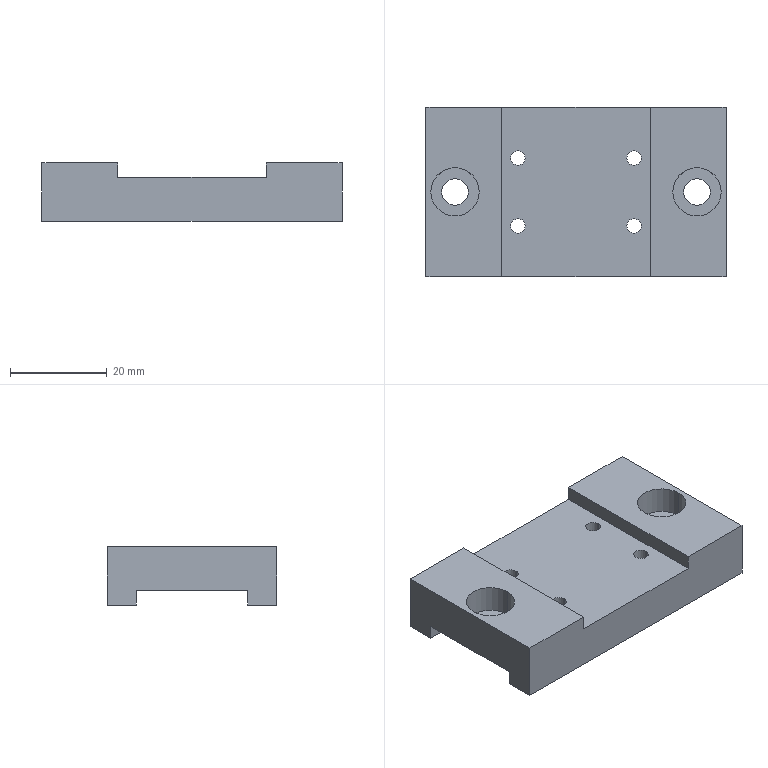Part | STEP file | X77-02302 | 1 solid | 32 faces | box 62 x 35 x 12 mm | volume 17327 mm3 | cylinder 16 | plane 16 | commonest cylinder face diameters 3 x8 5.5 x4 10 x4
STEP:
#1=CARTESIAN_POINT('',(-360.426,46.806,6.3));
#2=VERTEX_POINT('',#1);
#3=CARTESIAN_POINT('',(-350.426,46.806,6.3));
#4=VERTEX_POINT('',#3);
#5=CARTESIAN_POINT('',(-355.426,46.806,6.3));
#6=DIRECTION('',(0.,0.,1.));
#7=DIRECTION('',(1.,0.,0.));
#8=AXIS2_PLACEMENT_3D('',#5,#6,#7);
#9=CIRCLE('',#8,5.);
#10=EDGE_CURVE('',#2,#4,#9,.T.);
#11=ORIENTED_EDGE('',*,*,#10,.F.);
#12=CARTESIAN_POINT('',(-360.426,46.806,12.));
#13=VERTEX_POINT('',#12);
#14=CARTESIAN_POINT('',(-360.426,46.806,12.));
#15=DIRECTION('',(0.,0.,1.));
#16=VECTOR('',#15,1000.);
#17=LINE('',#14,#16);
#18=EDGE_CURVE('',#2,#13,#17,.T.);
#19=ORIENTED_EDGE('',*,*,#18,.T.);
#20=CARTESIAN_POINT('',(-350.426,46.806,12.));
#21=VERTEX_POINT('',#20);
#22=CARTESIAN_POINT('',(-355.426,46.806,12.));
#23=DIRECTION('',(0.,0.,1.));
#24=DIRECTION('',(1.,0.,0.));
#25=AXIS2_PLACEMENT_3D('',#22,#23,#24);
#26=CIRCLE('',#25,5.);
#27=EDGE_CURVE('',#13,#21,#26,.T.);
#28=ORIENTED_EDGE('',*,*,#27,.T.);
#29=CARTESIAN_POINT('',(-350.426,46.806,12.));
#30=DIRECTION('',(0.,0.,1.));
#31=VECTOR('',#30,1000.);
#32=LINE('',#29,#31);
#33=EDGE_CURVE('',#4,#21,#32,.T.);
#34=ORIENTED_EDGE('',*,*,#33,.F.);
#35=EDGE_LOOP('',(#11,#19,#28,#34));
#36=FACE_OUTER_BOUND('',#35,.T.);
#37=CARTESIAN_POINT('',(-355.426,46.806,12.));
#38=DIRECTION('',(0.,0.,1.));
#39=DIRECTION('',(1.,0.,0.));
#40=AXIS2_PLACEMENT_3D('',#37,#38,#39);
#41=CYLINDRICAL_SURFACE('',#40,5.);
#42=ADVANCED_FACE('',(#36),#41,.F.);
#43=CARTESIAN_POINT('',(-358.176,46.806,3.));
#44=VERTEX_POINT('',#43);
#45=CARTESIAN_POINT('',(-352.676,46.806,3.));
#46=VERTEX_POINT('',#45);
#47=CARTESIAN_POINT('',(-355.426,46.806,3.));
#48=DIRECTION('',(0.,0.,1.));
#49=DIRECTION('',(1.,0.,0.));
#50=AXIS2_PLACEMENT_3D('',#47,#48,#49);
#51=CIRCLE('',#50,2.75);
#52=EDGE_CURVE('',#44,#46,#51,.T.);
#53=ORIENTED_EDGE('',*,*,#52,.F.);
#54=CARTESIAN_POINT('',(-358.176,46.806,6.3));
#55=VERTEX_POINT('',#54);
#56=CARTESIAN_POINT('',(-358.176,46.806,12.));
#57=DIRECTION('',(0.,0.,1.));
#58=VECTOR('',#57,1000.);
#59=LINE('',#56,#58);
#60=EDGE_CURVE('',#44,#55,#59,.T.);
#61=ORIENTED_EDGE('',*,*,#60,.T.);
#62=CARTESIAN_POINT('',(-352.676,46.806,6.3));
#63=VERTEX_POINT('',#62);
#64=CARTESIAN_POINT('',(-355.426,46.806,6.3));
#65=DIRECTION('',(0.,0.,1.));
#66=DIRECTION('',(1.,0.,0.));
#67=AXIS2_PLACEMENT_3D('',#64,#65,#66);
#68=CIRCLE('',#67,2.75);
#69=EDGE_CURVE('',#55,#63,#68,.T.);
#70=ORIENTED_EDGE('',*,*,#69,.T.);
#71=CARTESIAN_POINT('',(-352.676,46.806,12.));
#72=DIRECTION('',(0.,0.,1.));
#73=VECTOR('',#72,1000.);
#74=LINE('',#71,#73);
#75=EDGE_CURVE('',#46,#63,#74,.T.);
#76=ORIENTED_EDGE('',*,*,#75,.F.);
#77=EDGE_LOOP('',(#53,#61,#70,#76));
#78=FACE_OUTER_BOUND('',#77,.T.);
#79=CARTESIAN_POINT('',(-355.426,46.806,12.));
#80=DIRECTION('',(0.,0.,1.));
#81=DIRECTION('',(1.,0.,0.));
#82=AXIS2_PLACEMENT_3D('',#79,#80,#81);
#83=CYLINDRICAL_SURFACE('',#82,2.75);
#84=ADVANCED_FACE('',(#78),#83,.F.);
#85=CARTESIAN_POINT('',(-310.426,46.806,6.3));
#86=VERTEX_POINT('',#85);
#87=CARTESIAN_POINT('',(-300.426,46.806,6.3));
#88=VERTEX_POINT('',#87);
#89=CARTESIAN_POINT('',(-305.426,46.806,6.3));
#90=DIRECTION('',(0.,0.,1.));
#91=DIRECTION('',(1.,0.,0.));
#92=AXIS2_PLACEMENT_3D('',#89,#90,#91);
#93=CIRCLE('',#92,5.);
#94=EDGE_CURVE('',#86,#88,#93,.T.);
#95=ORIENTED_EDGE('',*,*,#94,.F.);
#96=CARTESIAN_POINT('',(-310.426,46.806,12.));
#97=VERTEX_POINT('',#96);
#98=CARTESIAN_POINT('',(-310.426,46.806,12.));
#99=DIRECTION('',(0.,0.,1.));
#100=VECTOR('',#99,1000.);
#101=LINE('',#98,#100);
#102=EDGE_CURVE('',#86,#97,#101,.T.);
#103=ORIENTED_EDGE('',*,*,#102,.T.);
#104=CARTESIAN_POINT('',(-300.426,46.806,12.));
#105=VERTEX_POINT('',#104);
#106=CARTESIAN_POINT('',(-305.426,46.806,12.));
#107=DIRECTION('',(0.,0.,1.));
#108=DIRECTION('',(1.,0.,0.));
#109=AXIS2_PLACEMENT_3D('',#106,#107,#108);
#110=CIRCLE('',#109,5.);
#111=EDGE_CURVE('',#97,#105,#110,.T.);
#112=ORIENTED_EDGE('',*,*,#111,.T.);
#113=CARTESIAN_POINT('',(-300.426,46.806,12.));
#114=DIRECTION('',(0.,0.,1.));
#115=VECTOR('',#114,1000.);
#116=LINE('',#113,#115);
#117=EDGE_CURVE('',#88,#105,#116,.T.);
#118=ORIENTED_EDGE('',*,*,#117,.F.);
#119=EDGE_LOOP('',(#95,#103,#112,#118));
#120=FACE_OUTER_BOUND('',#119,.T.);
#121=CARTESIAN_POINT('',(-305.426,46.806,12.));
#122=DIRECTION('',(0.,0.,1.));
#123=DIRECTION('',(1.,0.,0.));
#124=AXIS2_PLACEMENT_3D('',#121,#122,#123);
#125=CYLINDRICAL_SURFACE('',#124,5.);
#126=ADVANCED_FACE('',(#120),#125,.F.);
#127=CARTESIAN_POINT('',(-308.176,46.806,3.));
#128=VERTEX_POINT('',#127);
#129=CARTESIAN_POINT('',(-302.676,46.806,3.));
#130=VERTEX_POINT('',#129);
#131=CARTESIAN_POINT('',(-305.426,46.806,3.));
#132=DIRECTION('',(0.,0.,1.));
#133=DIRECTION('',(1.,0.,0.));
#134=AXIS2_PLACEMENT_3D('',#131,#132,#133);
#135=CIRCLE('',#134,2.75);
#136=EDGE_CURVE('',#128,#130,#135,.T.);
#137=ORIENTED_EDGE('',*,*,#136,.F.);
#138=CARTESIAN_POINT('',(-308.176,46.806,6.3));
#139=VERTEX_POINT('',#138);
#140=CARTESIAN_POINT('',(-308.176,46.806,12.));
#141=DIRECTION('',(0.,0.,1.));
#142=VECTOR('',#141,1000.);
#143=LINE('',#140,#142);
#144=EDGE_CURVE('',#128,#139,#143,.T.);
#145=ORIENTED_EDGE('',*,*,#144,.T.);
#146=CARTESIAN_POINT('',(-302.676,46.806,6.3));
#147=VERTEX_POINT('',#146);
#148=CARTESIAN_POINT('',(-305.426,46.806,6.3));
#149=DIRECTION('',(0.,0.,1.));
#150=DIRECTION('',(1.,0.,0.));
#151=AXIS2_PLACEMENT_3D('',#148,#149,#150);
#152=CIRCLE('',#151,2.75);
#153=EDGE_CURVE('',#139,#147,#152,.T.);
#154=ORIENTED_EDGE('',*,*,#153,.T.);
#155=CARTESIAN_POINT('',(-302.676,46.806,12.));
#156=DIRECTION('',(0.,0.,1.));
#157=VECTOR('',#156,1000.);
#158=LINE('',#155,#157);
#159=EDGE_CURVE('',#130,#147,#158,.T.);
#160=ORIENTED_EDGE('',*,*,#159,.F.);
#161=EDGE_LOOP('',(#137,#145,#154,#160));
#162=FACE_OUTER_BOUND('',#161,.T.);
#163=CARTESIAN_POINT('',(-305.426,46.806,12.));
#164=DIRECTION('',(0.,0.,1.));
#165=DIRECTION('',(1.,0.,0.));
#166=AXIS2_PLACEMENT_3D('',#163,#164,#165);
#167=CYLINDRICAL_SURFACE('',#166,2.75);
#168=ADVANCED_FACE('',(#162),#167,.F.);
#169=CARTESIAN_POINT('',(-319.926,53.806,3.));
#170=VERTEX_POINT('',#169);
#171=CARTESIAN_POINT('',(-316.926,53.806,3.));
#172=VERTEX_POINT('',#171);
#173=CARTESIAN_POINT('',(-318.426,53.806,3.));
#174=DIRECTION('',(0.,0.,1.));
#175=DIRECTION('',(1.,0.,0.));
#176=AXIS2_PLACEMENT_3D('',#173,#174,#175);
#177=CIRCLE('',#176,1.5);
#178=EDGE_CURVE('',#170,#172,#177,.T.);
#179=ORIENTED_EDGE('',*,*,#178,.F.);
#180=CARTESIAN_POINT('',(-319.926,53.806,9.));
#181=VERTEX_POINT('',#180);
#182=CARTESIAN_POINT('',(-319.926,53.806,12.));
#183=DIRECTION('',(0.,0.,1.));
#184=VECTOR('',#183,1000.);
#185=LINE('',#182,#184);
#186=EDGE_CURVE('',#170,#181,#185,.T.);
#187=ORIENTED_EDGE('',*,*,#186,.T.);
#188=CARTESIAN_POINT('',(-316.926,53.806,9.));
#189=VERTEX_POINT('',#188);
#190=CARTESIAN_POINT('',(-318.426,53.806,9.));
#191=DIRECTION('',(0.,0.,1.));
#192=DIRECTION('',(1.,0.,0.));
#193=AXIS2_PLACEMENT_3D('',#190,#191,#192);
#194=CIRCLE('',#193,1.5);
#195=EDGE_CURVE('',#181,#189,#194,.T.);
#196=ORIENTED_EDGE('',*,*,#195,.T.);
#197=CARTESIAN_POINT('',(-316.926,53.806,12.));
#198=DIRECTION('',(0.,0.,1.));
#199=VECTOR('',#198,1000.);
#200=LINE('',#197,#199);
#201=EDGE_CURVE('',#172,#189,#200,.T.);
#202=ORIENTED_EDGE('',*,*,#201,.F.);
#203=EDGE_LOOP('',(#179,#187,#196,#202));
#204=FACE_OUTER_BOUND('',#203,.T.);
#205=CARTESIAN_POINT('',(-318.426,53.806,12.));
#206=DIRECTION('',(0.,0.,1.));
#207=DIRECTION('',(1.,0.,0.));
#208=AXIS2_PLACEMENT_3D('',#205,#206,#207);
#209=CYLINDRICAL_SURFACE('',#208,1.5);
#210=ADVANCED_FACE('',(#204),#209,.F.);
#211=CARTESIAN_POINT('',(-343.926,53.806,3.));
#212=VERTEX_POINT('',#211);
#213=CARTESIAN_POINT('',(-340.926,53.806,3.));
#214=VERTEX_POINT('',#213);
#215=CARTESIAN_POINT('',(-342.426,53.806,3.));
#216=DIRECTION('',(0.,0.,1.));
#217=DIRECTION('',(1.,0.,0.));
#218=AXIS2_PLACEMENT_3D('',#215,#216,#217);
#219=CIRCLE('',#218,1.5);
#220=EDGE_CURVE('',#212,#214,#219,.T.);
#221=ORIENTED_EDGE('',*,*,#220,.F.);
#222=CARTESIAN_POINT('',(-343.926,53.806,9.));
#223=VERTEX_POINT('',#222);
#224=CARTESIAN_POINT('',(-343.926,53.806,12.));
#225=DIRECTION('',(0.,0.,1.));
#226=VECTOR('',#225,1000.);
#227=LINE('',#224,#226);
#228=EDGE_CURVE('',#212,#223,#227,.T.);
#229=ORIENTED_EDGE('',*,*,#228,.T.);
#230=CARTESIAN_POINT('',(-340.926,53.806,9.));
#231=VERTEX_POINT('',#230);
#232=CARTESIAN_POINT('',(-342.426,53.806,9.));
#233=DIRECTION('',(0.,0.,1.));
#234=DIRECTION('',(1.,0.,0.));
#235=AXIS2_PLACEMENT_3D('',#232,#233,#234);
#236=CIRCLE('',#235,1.5);
#237=EDGE_CURVE('',#223,#231,#236,.T.);
#238=ORIENTED_EDGE('',*,*,#237,.T.);
#239=CARTESIAN_POINT('',(-340.926,53.806,12.));
#240=DIRECTION('',(0.,0.,1.));
#241=VECTOR('',#240,1000.);
#242=LINE('',#239,#241);
#243=EDGE_CURVE('',#214,#231,#242,.T.);
#244=ORIENTED_EDGE('',*,*,#243,.F.);
#245=EDGE_LOOP('',(#221,#229,#238,#244));
#246=FACE_OUTER_BOUND('',#245,.T.);
#247=CARTESIAN_POINT('',(-342.426,53.806,12.));
#248=DIRECTION('',(0.,0.,1.));
#249=DIRECTION('',(1.,0.,0.));
#250=AXIS2_PLACEMENT_3D('',#247,#248,#249);
#251=CYLINDRICAL_SURFACE('',#250,1.5);
#252=ADVANCED_FACE('',(#246),#251,.F.);
#253=CARTESIAN_POINT('',(-319.926,39.806,3.));
#254=VERTEX_POINT('',#253);
#255=CARTESIAN_POINT('',(-316.926,39.806,3.));
#256=VERTEX_POINT('',#255);
#257=CARTESIAN_POINT('',(-318.426,39.806,3.));
#258=DIRECTION('',(0.,0.,1.));
#259=DIRECTION('',(1.,0.,0.));
#260=AXIS2_PLACEMENT_3D('',#257,#258,#259);
#261=CIRCLE('',#260,1.5);
#262=EDGE_CURVE('',#254,#256,#261,.T.);
#263=ORIENTED_EDGE('',*,*,#262,.F.);
#264=CARTESIAN_POINT('',(-319.926,39.806,9.));
#265=VERTEX_POINT('',#264);
#266=CARTESIAN_POINT('',(-319.926,39.806,12.));
#267=DIRECTION('',(0.,0.,1.));
#268=VECTOR('',#267,1000.);
#269=LINE('',#266,#268);
#270=EDGE_CURVE('',#254,#265,#269,.T.);
#271=ORIENTED_EDGE('',*,*,#270,.T.);
#272=CARTESIAN_POINT('',(-316.926,39.806,9.));
#273=VERTEX_POINT('',#272);
#274=CARTESIAN_POINT('',(-318.426,39.806,9.));
#275=DIRECTION('',(0.,0.,1.));
#276=DIRECTION('',(1.,0.,0.));
#277=AXIS2_PLACEMENT_3D('',#274,#275,#276);
#278=CIRCLE('',#277,1.5);
#279=EDGE_CURVE('',#265,#273,#278,.T.);
#280=ORIENTED_EDGE('',*,*,#279,.T.);
#281=CARTESIAN_POINT('',(-316.926,39.806,12.));
#282=DIRECTION('',(0.,0.,1.));
#283=VECTOR('',#282,1000.);
#284=LINE('',#281,#283);
#285=EDGE_CURVE('',#256,#273,#284,.T.);
#286=ORIENTED_EDGE('',*,*,#285,.F.);
#287=EDGE_LOOP('',(#263,#271,#280,#286));
#288=FACE_OUTER_BOUND('',#287,.T.);
#289=CARTESIAN_POINT('',(-318.426,39.806,12.));
#290=DIRECTION('',(0.,0.,1.));
#291=DIRECTION('',(1.,0.,0.));
#292=AXIS2_PLACEMENT_3D('',#289,#290,#291);
#293=CYLINDRICAL_SURFACE('',#292,1.5);
#294=ADVANCED_FACE('',(#288),#293,.F.);
#295=CARTESIAN_POINT('',(-343.926,39.806,3.));
#296=VERTEX_POINT('',#295);
#297=CARTESIAN_POINT('',(-340.926,39.806,3.));
#298=VERTEX_POINT('',#297);
#299=CARTESIAN_POINT('',(-342.426,39.806,3.));
#300=DIRECTION('',(0.,0.,1.));
#301=DIRECTION('',(1.,0.,0.));
#302=AXIS2_PLACEMENT_3D('',#299,#300,#301);
#303=CIRCLE('',#302,1.5);
#304=EDGE_CURVE('',#296,#298,#303,.T.);
#305=ORIENTED_EDGE('',*,*,#304,.F.);
#306=CARTESIAN_POINT('',(-343.926,39.806,9.));
#307=VERTEX_POINT('',#306);
#308=CARTESIAN_POINT('',(-343.926,39.806,12.));
#309=DIRECTION('',(0.,0.,1.));
#310=VECTOR('',#309,1000.);
#311=LINE('',#308,#310);
#312=EDGE_CURVE('',#296,#307,#311,.T.);
#313=ORIENTED_EDGE('',*,*,#312,.T.);
#314=CARTESIAN_POINT('',(-340.926,39.806,9.));
#315=VERTEX_POINT('',#314);
#316=CARTESIAN_POINT('',(-342.426,39.806,9.));
#317=DIRECTION('',(0.,0.,1.));
#318=DIRECTION('',(1.,0.,0.));
#319=AXIS2_PLACEMENT_3D('',#316,#317,#318);
#320=CIRCLE('',#319,1.5);
#321=EDGE_CURVE('',#307,#315,#320,.T.);
#322=ORIENTED_EDGE('',*,*,#321,.T.);
#323=CARTESIAN_POINT('',(-340.926,39.806,12.));
#324=DIRECTION('',(0.,0.,1.));
#325=VECTOR('',#324,1000.);
#326=LINE('',#323,#325);
#327=EDGE_CURVE('',#298,#315,#326,.T.);
#328=ORIENTED_EDGE('',*,*,#327,.F.);
#329=EDGE_LOOP('',(#305,#313,#322,#328));
#330=FACE_OUTER_BOUND('',#329,.T.);
#331=CARTESIAN_POINT('',(-342.426,39.806,12.));
#332=DIRECTION('',(0.,0.,1.));
#333=DIRECTION('',(1.,0.,0.));
#334=AXIS2_PLACEMENT_3D('',#331,#332,#333);
#335=CYLINDRICAL_SURFACE('',#334,1.5);
#336=ADVANCED_FACE('',(#330),#335,.F.);
#337=CARTESIAN_POINT('',(-361.426,35.306,0.));
#338=VERTEX_POINT('',#337);
#339=CARTESIAN_POINT('',(-361.426,29.306,0.));
#340=VERTEX_POINT('',#339);
#341=CARTESIAN_POINT('',(-361.426,29.306,0.));
#342=DIRECTION('',(0.,-1.,0.));
#343=VECTOR('',#342,1000.);
#344=LINE('',#341,#343);
#345=EDGE_CURVE('',#338,#340,#344,.T.);
#346=ORIENTED_EDGE('',*,*,#345,.F.);
#347=CARTESIAN_POINT('',(-299.426,35.306,0.));
#348=VERTEX_POINT('',#347);
#349=CARTESIAN_POINT('',(-361.426,35.306,0.));
#350=DIRECTION('',(1.,0.,0.));
#351=VECTOR('',#350,1000.);
#352=LINE('',#349,#351);
#353=EDGE_CURVE('',#338,#348,#352,.T.);
#354=ORIENTED_EDGE('',*,*,#353,.T.);
#355=CARTESIAN_POINT('',(-299.426,29.306,0.));
#356=VERTEX_POINT('',#355);
#357=CARTESIAN_POINT('',(-299.426,29.306,0.));
#358=DIRECTION('',(0.,1.,0.));
#359=VECTOR('',#358,1000.);
#360=LINE('',#357,#359);
#361=EDGE_CURVE('',#356,#348,#360,.T.);
#362=ORIENTED_EDGE('',*,*,#361,.F.);
#363=CARTESIAN_POINT('',(-299.426,29.306,0.));
#364=DIRECTION('',(1.,0.,0.));
#365=VECTOR('',#364,1000.);
#366=LINE('',#363,#365);
#367=EDGE_CURVE('',#340,#356,#366,.T.);
#368=ORIENTED_EDGE('',*,*,#367,.F.);
#369=EDGE_LOOP('',(#346,#354,#362,#368));
#370=FACE_OUTER_BOUND('',#369,.T.);
#371=CARTESIAN_POINT('',(-361.426,64.306,0.));
#372=DIRECTION('',(0.,0.,1.));
#373=DIRECTION('',(1.,0.,0.));
#374=AXIS2_PLACEMENT_3D('',#371,#372,#373);
#375=PLANE('',#374);
#376=ADVANCED_FACE('',(#370),#375,.F.);
#377=CARTESIAN_POINT('',(-305.426,46.806,12.));
#378=DIRECTION('',(0.,0.,1.));
#379=DIRECTION('',(1.,0.,0.));
#380=AXIS2_PLACEMENT_3D('',#377,#378,#379);
#381=CIRCLE('',#380,5.);
#382=EDGE_CURVE('',#105,#97,#381,.T.);
#383=ORIENTED_EDGE('',*,*,#382,.F.);
#384=ORIENTED_EDGE('',*,*,#111,.F.);
#385=EDGE_LOOP('',(#383,#384));
#386=FACE_BOUND('',#385,.T.);
#387=CARTESIAN_POINT('',(-315.126,29.306,12.));
#388=VERTEX_POINT('',#387);
#389=CARTESIAN_POINT('',(-315.126,64.306,12.));
#390=VERTEX_POINT('',#389);
#391=CARTESIAN_POINT('',(-315.126,64.306,12.));
#392=DIRECTION('',(0.,1.,0.));
#393=VECTOR('',#392,1000.);
#394=LINE('',#391,#393);
#395=EDGE_CURVE('',#388,#390,#394,.T.);
#396=ORIENTED_EDGE('',*,*,#395,.F.);
#397=CARTESIAN_POINT('',(-299.426,29.306,12.));
#398=VERTEX_POINT('',#397);
#399=CARTESIAN_POINT('',(-299.426,29.306,12.));
#400=DIRECTION('',(1.,0.,0.));
#401=VECTOR('',#400,1000.);
#402=LINE('',#399,#401);
#403=EDGE_CURVE('',#388,#398,#402,.T.);
#404=ORIENTED_EDGE('',*,*,#403,.T.);
#405=CARTESIAN_POINT('',(-299.426,64.306,12.));
#406=VERTEX_POINT('',#405);
#407=CARTESIAN_POINT('',(-299.426,29.306,12.));
#408=DIRECTION('',(0.,1.,0.));
#409=VECTOR('',#408,1000.);
#410=LINE('',#407,#409);
#411=EDGE_CURVE('',#398,#406,#410,.T.);
#412=ORIENTED_EDGE('',*,*,#411,.T.);
#413=CARTESIAN_POINT('',(-299.426,64.306,12.));
#414=DIRECTION('',(-1.,0.,0.));
#415=VECTOR('',#414,1000.);
#416=LINE('',#413,#415);
#417=EDGE_CURVE('',#406,#390,#416,.T.);
#418=ORIENTED_EDGE('',*,*,#417,.T.);
#419=EDGE_LOOP('',(#396,#404,#412,#418));
#420=FACE_OUTER_BOUND('',#419,.T.);
#421=CARTESIAN_POINT('',(-361.426,64.306,12.));
#422=DIRECTION('',(0.,0.,1.));
#423=DIRECTION('',(1.,0.,0.));
#424=AXIS2_PLACEMENT_3D('',#421,#422,#423);
#425=PLANE('',#424);
#426=ADVANCED_FACE('',(#386,#420),#425,.T.);
#427=CARTESIAN_POINT('',(-361.426,58.306,3.));
#428=VERTEX_POINT('',#427);
#429=CARTESIAN_POINT('',(-361.426,35.306,3.));
#430=VERTEX_POINT('',#429);
#431=CARTESIAN_POINT('',(-361.426,35.306,3.));
#432=DIRECTION('',(0.,-1.,0.));
#433=VECTOR('',#432,1000.);
#434=LINE('',#431,#433);
#435=EDGE_CURVE('',#428,#430,#434,.T.);
#436=ORIENTED_EDGE('',*,*,#435,.T.);
#437=CARTESIAN_POINT('',(-361.426,35.306,0.));
#438=DIRECTION('',(0.,0.,-1.));
#439=VECTOR('',#438,1000.);
#440=LINE('',#437,#439);
#441=EDGE_CURVE('',#430,#338,#440,.T.);
#442=ORIENTED_EDGE('',*,*,#441,.T.);
#443=ORIENTED_EDGE('',*,*,#345,.T.);
#444=CARTESIAN_POINT('',(-361.426,29.306,12.));
#445=VERTEX_POINT('',#444);
#446=CARTESIAN_POINT('',(-361.426,29.306,12.));
#447=DIRECTION('',(0.,0.,-1.));
#448=VECTOR('',#447,1000.);
#449=LINE('',#446,#448);
#450=EDGE_CURVE('',#445,#340,#449,.T.);
#451=ORIENTED_EDGE('',*,*,#450,.F.);
#452=CARTESIAN_POINT('',(-361.426,64.306,12.));
#453=VERTEX_POINT('',#452);
#454=CARTESIAN_POINT('',(-361.426,29.306,12.));
#455=DIRECTION('',(0.,-1.,0.));
#456=VECTOR('',#455,1000.);
#457=LINE('',#454,#456);
#458=EDGE_CURVE('',#453,#445,#457,.T.);
#459=ORIENTED_EDGE('',*,*,#458,.F.);
#460=CARTESIAN_POINT('',(-361.426,64.306,0.));
#461=VERTEX_POINT('',#460);
#462=CARTESIAN_POINT('',(-361.426,64.306,12.));
#463=DIRECTION('',(0.,0.,-1.));
#464=VECTOR('',#463,1000.);
#465=LINE('',#462,#464);
#466=EDGE_CURVE('',#453,#461,#465,.T.);
#467=ORIENTED_EDGE('',*,*,#466,.T.);
#468=CARTESIAN_POINT('',(-361.426,58.306,0.));
#469=VERTEX_POINT('',#468);
#470=CARTESIAN_POINT('',(-361.426,29.306,0.));
#471=DIRECTION('',(0.,-1.,0.));
#472=VECTOR('',#471,1000.);
#473=LINE('',#470,#472);
#474=EDGE_CURVE('',#461,#469,#473,.T.);
#475=ORIENTED_EDGE('',*,*,#474,.T.);
#476=CARTESIAN_POINT('',(-361.426,58.306,0.));
#477=DIRECTION('',(0.,0.,1.));
#478=VECTOR('',#477,1000.);
#479=LINE('',#476,#478);
#480=EDGE_CURVE('',#469,#428,#479,.T.);
#481=ORIENTED_EDGE('',*,*,#480,.T.);
#482=EDGE_LOOP('',(#436,#442,#443,#451,#459,#467,#475,#481));
#483=FACE_OUTER_BOUND('',#482,.T.);
#484=CARTESIAN_POINT('',(-361.426,29.306,12.));
#485=DIRECTION('',(1.,0.,0.));
#486=DIRECTION('',(0.,0.,-1.));
#487=AXIS2_PLACEMENT_3D('',#484,#485,#486);
#488=PLANE('',#487);
#489=ADVANCED_FACE('',(#483),#488,.F.);
#490=ORIENTED_EDGE('',*,*,#403,.F.);
#491=CARTESIAN_POINT('',(-315.126,29.306,9.));
#492=VERTEX_POINT('',#491);
#493=CARTESIAN_POINT('',(-315.126,29.306,12.));
#494=DIRECTION('',(0.,0.,-1.));
#495=VECTOR('',#494,1000.);
#496=LINE('',#493,#495);
#497=EDGE_CURVE('',#388,#492,#496,.T.);
#498=ORIENTED_EDGE('',*,*,#497,.T.);
#499=CARTESIAN_POINT('',(-345.726,29.306,9.));
#500=VERTEX_POINT('',#499);
#501=CARTESIAN_POINT('',(-299.426,29.306,9.));
#502=DIRECTION('',(1.,0.,0.));
#503=VECTOR('',#502,1000.);
#504=LINE('',#501,#503);
#505=EDGE_CURVE('',#500,#492,#504,.T.);
#506=ORIENTED_EDGE('',*,*,#505,.F.);
#507=CARTESIAN_POINT('',(-345.726,29.306,12.));
#508=VERTEX_POINT('',#507);
#509=CARTESIAN_POINT('',(-345.726,29.306,12.));
#510=DIRECTION('',(0.,0.,1.));
#511=VECTOR('',#510,1000.);
#512=LINE('',#509,#511);
#513=EDGE_CURVE('',#500,#508,#512,.T.);
#514=ORIENTED_EDGE('',*,*,#513,.T.);
#515=CARTESIAN_POINT('',(-299.426,29.306,12.));
#516=DIRECTION('',(1.,0.,0.));
#517=VECTOR('',#516,1000.);
#518=LINE('',#515,#517);
#519=EDGE_CURVE('',#445,#508,#518,.T.);
#520=ORIENTED_EDGE('',*,*,#519,.F.);
#521=ORIENTED_EDGE('',*,*,#450,.T.);
#522=ORIENTED_EDGE('',*,*,#367,.T.);
#523=CARTESIAN_POINT('',(-299.426,29.306,12.));
#524=DIRECTION('',(0.,0.,-1.));
#525=VECTOR('',#524,1000.);
#526=LINE('',#523,#525);
#527=EDGE_CURVE('',#398,#356,#526,.T.);
#528=ORIENTED_EDGE('',*,*,#527,.F.);
#529=EDGE_LOOP('',(#490,#498,#506,#514,#520,#521,#522,#528));
#530=FACE_OUTER_BOUND('',#529,.T.);
#531=CARTESIAN_POINT('',(-299.426,29.306,12.));
#532=DIRECTION('',(0.,1.,0.));
#533=DIRECTION('',(-1.,0.,0.));
#534=AXIS2_PLACEMENT_3D('',#531,#532,#533);
#535=PLANE('',#534);
#536=ADVANCED_FACE('',(#530),#535,.F.);
#537=ORIENTED_EDGE('',*,*,#361,.T.);
#538=CARTESIAN_POINT('',(-299.426,35.306,3.));
#539=VERTEX_POINT('',#538);
#540=CARTESIAN_POINT('',(-299.426,35.306,0.));
#541=DIRECTION('',(0.,0.,-1.));
#542=VECTOR('',#541,1000.);
#543=LINE('',#540,#542);
#544=EDGE_CURVE('',#539,#348,#543,.T.);
#545=ORIENTED_EDGE('',*,*,#544,.F.);
#546=CARTESIAN_POINT('',(-299.426,58.306,3.));
#547=VERTEX_POINT('',#546);
#548=CARTESIAN_POINT('',(-299.426,35.306,3.));
#549=DIRECTION('',(0.,-1.,0.));
#550=VECTOR('',#549,1000.);
#551=LINE('',#548,#550);
#552=EDGE_CURVE('',#547,#539,#551,.T.);
#553=ORIENTED_EDGE('',*,*,#552,.F.);
#554=CARTESIAN_POINT('',(-299.426,58.306,0.));
#555=VERTEX_POINT('',#554);
#556=CARTESIAN_POINT('',(-299.426,58.306,0.));
#557=DIRECTION('',(0.,0.,1.));
#558=VECTOR('',#557,1000.);
#559=LINE('',#556,#558);
#560=EDGE_CURVE('',#555,#547,#559,.T.);
#561=ORIENTED_EDGE('',*,*,#560,.F.);
#562=CARTESIAN_POINT('',(-299.426,64.306,0.));
#563=VERTEX_POINT('',#562);
#564=CARTESIAN_POINT('',(-299.426,29.306,0.));
#565=DIRECTION('',(0.,1.,0.));
#566=VECTOR('',#565,1000.);
#567=LINE('',#564,#566);
#568=EDGE_CURVE('',#555,#563,#567,.T.);
#569=ORIENTED_EDGE('',*,*,#568,.T.);
#570=CARTESIAN_POINT('',(-299.426,64.306,12.));
#571=DIRECTION('',(0.,0.,-1.));
#572=VECTOR('',#571,1000.);
#573=LINE('',#570,#572);
#574=EDGE_CURVE('',#406,#563,#573,.T.);
#575=ORIENTED_EDGE('',*,*,#574,.F.);
#576=ORIENTED_EDGE('',*,*,#411,.F.);
#577=ORIENTED_EDGE('',*,*,#527,.T.);
#578=EDGE_LOOP('',(#537,#545,#553,#561,#569,#575,#576,#577));
#579=FACE_OUTER_BOUND('',#578,.T.);
#580=CARTESIAN_POINT('',(-299.426,29.306,12.));
#581=DIRECTION('',(-1.,0.,0.));
#582=DIRECTION('',(0.,0.,1.));
#583=AXIS2_PLACEMENT_3D('',#580,#581,#582);
#584=PLANE('',#583);
#585=ADVANCED_FACE('',(#579),#584,.F.);
#586=CARTESIAN_POINT('',(-315.126,64.306,9.));
#587=VERTEX_POINT('',#586);
#588=CARTESIAN_POINT('',(-345.726,64.306,9.));
#589=VERTEX_POINT('',#588);
#590=CARTESIAN_POINT('',(-299.426,64.306,9.));
#591=DIRECTION('',(-1.,0.,0.));
#592=VECTOR('',#591,1000.);
#593=LINE('',#590,#592);
#594=EDGE_CURVE('',#587,#589,#593,.T.);
#595=ORIENTED_EDGE('',*,*,#594,.F.);
#596=CARTESIAN_POINT('',(-315.126,64.306,12.));
#597=DIRECTION('',(0.,0.,1.));
#598=VECTOR('',#597,1000.);
#599=LINE('',#596,#598);
#600=EDGE_CURVE('',#587,#390,#599,.T.);
#601=ORIENTED_EDGE('',*,*,#600,.T.);
#602=ORIENTED_EDGE('',*,*,#417,.F.);
#603=ORIENTED_EDGE('',*,*,#574,.T.);
#604=CARTESIAN_POINT('',(-299.426,64.306,0.));
#605=DIRECTION('',(-1.,0.,0.));
#606=VECTOR('',#605,1000.);
#607=LINE('',#604,#606);
#608=EDGE_CURVE('',#563,#461,#607,.T.);
#609=ORIENTED_EDGE('',*,*,#608,.T.);
#610=ORIENTED_EDGE('',*,*,#466,.F.);
#611=CARTESIAN_POINT('',(-345.726,64.306,12.));
#612=VERTEX_POINT('',#611);
#613=CARTESIAN_POINT('',(-299.426,64.306,12.));
#614=DIRECTION('',(-1.,0.,0.));
#615=VECTOR('',#614,1000.);
#616=LINE('',#613,#615);
#617=EDGE_CURVE('',#612,#453,#616,.T.);
#618=ORIENTED_EDGE('',*,*,#617,.F.);
#619=CARTESIAN_POINT('',(-345.726,64.306,12.));
#620=DIRECTION('',(0.,0.,-1.));
#621=VECTOR('',#620,1000.);
#622=LINE('',#619,#621);
#623=EDGE_CURVE('',#612,#589,#622,.T.);
#624=ORIENTED_EDGE('',*,*,#623,.T.);
#625=EDGE_LOOP('',(#595,#601,#602,#603,#609,#610,#618,#624));
#626=FACE_OUTER_BOUND('',#625,.T.);
#627=CARTESIAN_POINT('',(-299.426,64.306,12.));
#628=DIRECTION('',(0.,-1.,0.));
#629=DIRECTION('',(0.,0.,-1.));
#630=AXIS2_PLACEMENT_3D('',#627,#628,#629);
#631=PLANE('',#630);
#632=ADVANCED_FACE('',(#626),#631,.F.);
#633=CARTESIAN_POINT('',(-355.426,46.806,12.));
#634=DIRECTION('',(0.,0.,1.));
#635=DIRECTION('',(1.,0.,0.));
#636=AXIS2_PLACEMENT_3D('',#633,#634,#635);
#637=CIRCLE('',#636,5.);
#638=EDGE_CURVE('',#21,#13,#637,.T.);
#639=ORIENTED_EDGE('',*,*,#638,.F.);
#640=ORIENTED_EDGE('',*,*,#27,.F.);
#641=EDGE_LOOP('',(#639,#640));
#642=FACE_BOUND('',#641,.T.);
#643=CARTESIAN_POINT('',(-345.726,64.306,12.));
#644=DIRECTION('',(0.,-1.,0.));
#645=VECTOR('',#644,1000.);
#646=LINE('',#643,#645);
#647=EDGE_CURVE('',#612,#508,#646,.T.);
#648=ORIENTED_EDGE('',*,*,#647,.F.);
#649=ORIENTED_EDGE('',*,*,#617,.T.);
#650=ORIENTED_EDGE('',*,*,#458,.T.);
#651=ORIENTED_EDGE('',*,*,#519,.T.);
#652=EDGE_LOOP('',(#648,#649,#650,#651));
#653=FACE_OUTER_BOUND('',#652,.T.);
#654=CARTESIAN_POINT('',(-361.426,64.306,12.));
#655=DIRECTION('',(0.,0.,1.));
#656=DIRECTION('',(1.,0.,0.));
#657=AXIS2_PLACEMENT_3D('',#654,#655,#656);
#658=PLANE('',#657);
#659=ADVANCED_FACE('',(#642,#653),#658,.T.);
#660=ORIENTED_EDGE('',*,*,#568,.F.);
#661=CARTESIAN_POINT('',(-361.426,58.306,0.));
#662=DIRECTION('',(1.,0.,0.));
#663=VECTOR('',#662,1000.);
#664=LINE('',#661,#663);
#665=EDGE_CURVE('',#469,#555,#664,.T.);
#666=ORIENTED_EDGE('',*,*,#665,.F.);
#667=ORIENTED_EDGE('',*,*,#474,.F.);
#668=ORIENTED_EDGE('',*,*,#608,.F.);
#669=EDGE_LOOP('',(#660,#666,#667,#668));
#670=FACE_OUTER_BOUND('',#669,.T.);
#671=CARTESIAN_POINT('',(-361.426,64.306,0.));
#672=DIRECTION('',(0.,0.,1.));
#673=DIRECTION('',(1.,0.,0.));
#674=AXIS2_PLACEMENT_3D('',#671,#672,#673);
#675=PLANE('',#674);
#676=ADVANCED_FACE('',(#670),#675,.F.);
#677=CARTESIAN_POINT('',(-318.426,53.806,9.));
#678=DIRECTION('',(0.,0.,1.));
#679=DIRECTION('',(1.,0.,0.));
#680=AXIS2_PLACEMENT_3D('',#677,#678,#679);
#681=CIRCLE('',#680,1.5);
#682=EDGE_CURVE('',#189,#181,#681,.T.);
#683=ORIENTED_EDGE('',*,*,#682,.F.);
#684=ORIENTED_EDGE('',*,*,#195,.F.);
#685=EDGE_LOOP('',(#683,#684));
#686=FACE_BOUND('',#685,.T.);
#687=CARTESIAN_POINT('',(-342.426,53.806,9.));
#688=DIRECTION('',(0.,0.,1.));
#689=DIRECTION('',(1.,0.,0.));
#690=AXIS2_PLACEMENT_3D('',#687,#688,#689);
#691=CIRCLE('',#690,1.5);
#692=EDGE_CURVE('',#231,#223,#691,.T.);
#693=ORIENTED_EDGE('',*,*,#692,.F.);
#694=ORIENTED_EDGE('',*,*,#237,.F.);
#695=EDGE_LOOP('',(#693,#694));
#696=FACE_BOUND('',#695,.T.);
#697=CARTESIAN_POINT('',(-318.426,39.806,9.));
#698=DIRECTION('',(0.,0.,1.));
#699=DIRECTION('',(1.,0.,0.));
#700=AXIS2_PLACEMENT_3D('',#697,#698,#699);
#701=CIRCLE('',#700,1.5);
#702=EDGE_CURVE('',#273,#265,#701,.T.);
#703=ORIENTED_EDGE('',*,*,#702,.F.);
#704=ORIENTED_EDGE('',*,*,#279,.F.);
#705=EDGE_LOOP('',(#703,#704));
#706=FACE_BOUND('',#705,.T.);
#707=CARTESIAN_POINT('',(-342.426,39.806,9.));
#708=DIRECTION('',(0.,0.,1.));
#709=DIRECTION('',(1.,0.,0.));
#710=AXIS2_PLACEMENT_3D('',#707,#708,#709);
#711=CIRCLE('',#710,1.5);
#712=EDGE_CURVE('',#315,#307,#711,.T.);
#713=ORIENTED_EDGE('',*,*,#712,.F.);
#714=ORIENTED_EDGE('',*,*,#321,.F.);
#715=EDGE_LOOP('',(#713,#714));
#716=FACE_BOUND('',#715,.T.);
#717=ORIENTED_EDGE('',*,*,#505,.T.);
#718=CARTESIAN_POINT('',(-315.126,22.306,9.));
#719=DIRECTION('',(0.,1.,0.));
#720=VECTOR('',#719,1000.);
#721=LINE('',#718,#720);
#722=EDGE_CURVE('',#492,#587,#721,.T.);
#723=ORIENTED_EDGE('',*,*,#722,.T.);
#724=ORIENTED_EDGE('',*,*,#594,.T.);
#725=CARTESIAN_POINT('',(-345.726,22.306,9.));
#726=DIRECTION('',(0.,-1.,0.));
#727=VECTOR('',#726,1000.);
#728=LINE('',#725,#727);
#729=EDGE_CURVE('',#589,#500,#728,.T.);
#730=ORIENTED_EDGE('',*,*,#729,.T.);
#731=EDGE_LOOP('',(#717,#723,#724,#730));
#732=FACE_OUTER_BOUND('',#731,.T.);
#733=CARTESIAN_POINT('',(-315.126,69.516,9.));
#734=DIRECTION('',(0.,0.,1.));
#735=DIRECTION('',(1.,0.,0.));
#736=AXIS2_PLACEMENT_3D('',#733,#734,#735);
#737=PLANE('',#736);
#738=ADVANCED_FACE('',(#686,#696,#706,#716,#732),#737,.T.);
#739=ORIENTED_EDGE('',*,*,#395,.T.);
#740=ORIENTED_EDGE('',*,*,#600,.F.);
#741=ORIENTED_EDGE('',*,*,#722,.F.);
#742=ORIENTED_EDGE('',*,*,#497,.F.);
#743=EDGE_LOOP('',(#739,#740,#741,#742));
#744=FACE_OUTER_BOUND('',#743,.T.);
#745=CARTESIAN_POINT('',(-315.126,22.306,9.));
#746=DIRECTION('',(1.,0.,0.));
#747=DIRECTION('',(0.,0.,-1.));
#748=AXIS2_PLACEMENT_3D('',#745,#746,#747);
#749=PLANE('',#748);
#750=ADVANCED_FACE('',(#744),#749,.F.);
#751=ORIENTED_EDGE('',*,*,#729,.F.);
#752=ORIENTED_EDGE('',*,*,#623,.F.);
#753=ORIENTED_EDGE('',*,*,#647,.T.);
#754=ORIENTED_EDGE('',*,*,#513,.F.);
#755=EDGE_LOOP('',(#751,#752,#753,#754));
#756=FACE_OUTER_BOUND('',#755,.T.);
#757=CARTESIAN_POINT('',(-345.726,22.306,9.));
#758=DIRECTION('',(-1.,0.,0.));
#759=DIRECTION('',(0.,0.,1.));
#760=AXIS2_PLACEMENT_3D('',#757,#758,#759);
#761=PLANE('',#760);
#762=ADVANCED_FACE('',(#756),#761,.F.);
#763=ORIENTED_EDGE('',*,*,#544,.T.);
#764=ORIENTED_EDGE('',*,*,#353,.F.);
#765=ORIENTED_EDGE('',*,*,#441,.F.);
#766=CARTESIAN_POINT('',(-361.426,35.306,3.));
#767=DIRECTION('',(1.,0.,0.));
#768=VECTOR('',#767,1000.);
#769=LINE('',#766,#768);
#770=EDGE_CURVE('',#430,#539,#769,.T.);
#771=ORIENTED_EDGE('',*,*,#770,.T.);
#772=EDGE_LOOP('',(#763,#764,#765,#771));
#773=FACE_OUTER_BOUND('',#772,.T.);
#774=CARTESIAN_POINT('',(-361.426,35.306,0.));
#775=DIRECTION('',(0.,-1.,0.));
#776=DIRECTION('',(0.,0.,-1.));
#777=AXIS2_PLACEMENT_3D('',#774,#775,#776);
#778=PLANE('',#777);
#779=ADVANCED_FACE('',(#773),#778,.F.);
#780=CARTESIAN_POINT('',(-355.426,46.806,3.));
#781=DIRECTION('',(0.,0.,1.));
#782=DIRECTION('',(1.,0.,0.));
#783=AXIS2_PLACEMENT_3D('',#780,#781,#782);
#784=CIRCLE('',#783,2.75);
#785=EDGE_CURVE('',#46,#44,#784,.T.);
#786=ORIENTED_EDGE('',*,*,#785,.T.);
#787=ORIENTED_EDGE('',*,*,#52,.T.);
#788=EDGE_LOOP('',(#786,#787));
#789=FACE_BOUND('',#788,.T.);
#790=CARTESIAN_POINT('',(-305.426,46.806,3.));
#791=DIRECTION('',(0.,0.,1.));
#792=DIRECTION('',(1.,0.,0.));
#793=AXIS2_PLACEMENT_3D('',#790,#791,#792);
#794=CIRCLE('',#793,2.75);
#795=EDGE_CURVE('',#130,#128,#794,.T.);
#796=ORIENTED_EDGE('',*,*,#795,.T.);
#797=ORIENTED_EDGE('',*,*,#136,.T.);
#798=EDGE_LOOP('',(#796,#797));
#799=FACE_BOUND('',#798,.T.);
#800=CARTESIAN_POINT('',(-318.426,53.806,3.));
#801=DIRECTION('',(0.,0.,1.));
#802=DIRECTION('',(1.,0.,0.));
#803=AXIS2_PLACEMENT_3D('',#800,#801,#802);
#804=CIRCLE('',#803,1.5);
#805=EDGE_CURVE('',#172,#170,#804,.T.);
#806=ORIENTED_EDGE('',*,*,#805,.T.);
#807=ORIENTED_EDGE('',*,*,#178,.T.);
#808=EDGE_LOOP('',(#806,#807));
#809=FACE_BOUND('',#808,.T.);
#810=CARTESIAN_POINT('',(-342.426,53.806,3.));
#811=DIRECTION('',(0.,0.,1.));
#812=DIRECTION('',(1.,0.,0.));
#813=AXIS2_PLACEMENT_3D('',#810,#811,#812);
#814=CIRCLE('',#813,1.5);
#815=EDGE_CURVE('',#214,#212,#814,.T.);
#816=ORIENTED_EDGE('',*,*,#815,.T.);
#817=ORIENTED_EDGE('',*,*,#220,.T.);
#818=EDGE_LOOP('',(#816,#817));
#819=FACE_BOUND('',#818,.T.);
#820=CARTESIAN_POINT('',(-318.426,39.806,3.));
#821=DIRECTION('',(0.,0.,1.));
#822=DIRECTION('',(1.,0.,0.));
#823=AXIS2_PLACEMENT_3D('',#820,#821,#822);
#824=CIRCLE('',#823,1.5);
#825=EDGE_CURVE('',#256,#254,#824,.T.);
#826=ORIENTED_EDGE('',*,*,#825,.T.);
#827=ORIENTED_EDGE('',*,*,#262,.T.);
#828=EDGE_LOOP('',(#826,#827));
#829=FACE_BOUND('',#828,.T.);
#830=CARTESIAN_POINT('',(-342.426,39.806,3.));
#831=DIRECTION('',(0.,0.,1.));
#832=DIRECTION('',(1.,0.,0.));
#833=AXIS2_PLACEMENT_3D('',#830,#831,#832);
#834=CIRCLE('',#833,1.5);
#835=EDGE_CURVE('',#298,#296,#834,.T.);
#836=ORIENTED_EDGE('',*,*,#835,.T.);
#837=ORIENTED_EDGE('',*,*,#304,.T.);
#838=EDGE_LOOP('',(#836,#837));
#839=FACE_BOUND('',#838,.T.);
#840=ORIENTED_EDGE('',*,*,#552,.T.);
#841=ORIENTED_EDGE('',*,*,#770,.F.);
#842=ORIENTED_EDGE('',*,*,#435,.F.);
#843=CARTESIAN_POINT('',(-361.426,58.306,3.));
#844=DIRECTION('',(1.,0.,0.));
#845=VECTOR('',#844,1000.);
#846=LINE('',#843,#845);
#847=EDGE_CURVE('',#428,#547,#846,.T.);
#848=ORIENTED_EDGE('',*,*,#847,.T.);
#849=EDGE_LOOP('',(#840,#841,#842,#848));
#850=FACE_OUTER_BOUND('',#849,.T.);
#851=CARTESIAN_POINT('',(-361.426,35.306,3.));
#852=DIRECTION('',(0.,0.,1.));
#853=DIRECTION('',(1.,0.,0.));
#854=AXIS2_PLACEMENT_3D('',#851,#852,#853);
#855=PLANE('',#854);
#856=ADVANCED_FACE('',(#789,#799,#809,#819,#829,#839,#850),#855,.F.);
#857=ORIENTED_EDGE('',*,*,#560,.T.);
#858=ORIENTED_EDGE('',*,*,#847,.F.);
#859=ORIENTED_EDGE('',*,*,#480,.F.);
#860=ORIENTED_EDGE('',*,*,#665,.T.);
#861=EDGE_LOOP('',(#857,#858,#859,#860));
#862=FACE_OUTER_BOUND('',#861,.T.);
#863=CARTESIAN_POINT('',(-361.426,58.306,0.));
#864=DIRECTION('',(0.,1.,0.));
#865=DIRECTION('',(0.,0.,1.));
#866=AXIS2_PLACEMENT_3D('',#863,#864,#865);
#867=PLANE('',#866);
#868=ADVANCED_FACE('',(#862),#867,.F.);
#869=ORIENTED_EDGE('',*,*,#312,.F.);
#870=ORIENTED_EDGE('',*,*,#835,.F.);
#871=ORIENTED_EDGE('',*,*,#327,.T.);
#872=ORIENTED_EDGE('',*,*,#712,.T.);
#873=EDGE_LOOP('',(#869,#870,#871,#872));
#874=FACE_OUTER_BOUND('',#873,.T.);
#875=CARTESIAN_POINT('',(-342.426,39.806,12.));
#876=DIRECTION('',(0.,0.,1.));
#877=DIRECTION('',(1.,0.,0.));
#878=AXIS2_PLACEMENT_3D('',#875,#876,#877);
#879=CYLINDRICAL_SURFACE('',#878,1.5);
#880=ADVANCED_FACE('',(#874),#879,.F.);
#881=ORIENTED_EDGE('',*,*,#270,.F.);
#882=ORIENTED_EDGE('',*,*,#825,.F.);
#883=ORIENTED_EDGE('',*,*,#285,.T.);
#884=ORIENTED_EDGE('',*,*,#702,.T.);
#885=EDGE_LOOP('',(#881,#882,#883,#884));
#886=FACE_OUTER_BOUND('',#885,.T.);
#887=CARTESIAN_POINT('',(-318.426,39.806,12.));
#888=DIRECTION('',(0.,0.,1.));
#889=DIRECTION('',(1.,0.,0.));
#890=AXIS2_PLACEMENT_3D('',#887,#888,#889);
#891=CYLINDRICAL_SURFACE('',#890,1.5);
#892=ADVANCED_FACE('',(#886),#891,.F.);
#893=ORIENTED_EDGE('',*,*,#228,.F.);
#894=ORIENTED_EDGE('',*,*,#815,.F.);
#895=ORIENTED_EDGE('',*,*,#243,.T.);
#896=ORIENTED_EDGE('',*,*,#692,.T.);
#897=EDGE_LOOP('',(#893,#894,#895,#896));
#898=FACE_OUTER_BOUND('',#897,.T.);
#899=CARTESIAN_POINT('',(-342.426,53.806,12.));
#900=DIRECTION('',(0.,0.,1.));
#901=DIRECTION('',(1.,0.,0.));
#902=AXIS2_PLACEMENT_3D('',#899,#900,#901);
#903=CYLINDRICAL_SURFACE('',#902,1.5);
#904=ADVANCED_FACE('',(#898),#903,.F.);
#905=ORIENTED_EDGE('',*,*,#186,.F.);
#906=ORIENTED_EDGE('',*,*,#805,.F.);
#907=ORIENTED_EDGE('',*,*,#201,.T.);
#908=ORIENTED_EDGE('',*,*,#682,.T.);
#909=EDGE_LOOP('',(#905,#906,#907,#908));
#910=FACE_OUTER_BOUND('',#909,.T.);
#911=CARTESIAN_POINT('',(-318.426,53.806,12.));
#912=DIRECTION('',(0.,0.,1.));
#913=DIRECTION('',(1.,0.,0.));
#914=AXIS2_PLACEMENT_3D('',#911,#912,#913);
#915=CYLINDRICAL_SURFACE('',#914,1.5);
#916=ADVANCED_FACE('',(#910),#915,.F.);
#917=ORIENTED_EDGE('',*,*,#144,.F.);
#918=ORIENTED_EDGE('',*,*,#795,.F.);
#919=ORIENTED_EDGE('',*,*,#159,.T.);
#920=CARTESIAN_POINT('',(-305.426,46.806,6.3));
#921=DIRECTION('',(0.,0.,1.));
#922=DIRECTION('',(1.,0.,0.));
#923=AXIS2_PLACEMENT_3D('',#920,#921,#922);
#924=CIRCLE('',#923,2.75);
#925=EDGE_CURVE('',#147,#139,#924,.T.);
#926=ORIENTED_EDGE('',*,*,#925,.T.);
#927=EDGE_LOOP('',(#917,#918,#919,#926));
#928=FACE_OUTER_BOUND('',#927,.T.);
#929=CARTESIAN_POINT('',(-305.426,46.806,12.));
#930=DIRECTION('',(0.,0.,1.));
#931=DIRECTION('',(1.,0.,0.));
#932=AXIS2_PLACEMENT_3D('',#929,#930,#931);
#933=CYLINDRICAL_SURFACE('',#932,2.75);
#934=ADVANCED_FACE('',(#928),#933,.F.);
#935=ORIENTED_EDGE('',*,*,#925,.F.);
#936=ORIENTED_EDGE('',*,*,#153,.F.);
#937=EDGE_LOOP('',(#935,#936));
#938=FACE_BOUND('',#937,.T.);
#939=CARTESIAN_POINT('',(-305.426,46.806,6.3));
#940=DIRECTION('',(0.,0.,1.));
#941=DIRECTION('',(1.,0.,0.));
#942=AXIS2_PLACEMENT_3D('',#939,#940,#941);
#943=CIRCLE('',#942,5.);
#944=EDGE_CURVE('',#88,#86,#943,.T.);
#945=ORIENTED_EDGE('',*,*,#944,.T.);
#946=ORIENTED_EDGE('',*,*,#94,.T.);
#947=EDGE_LOOP('',(#945,#946));
#948=FACE_OUTER_BOUND('',#947,.T.);
#949=CARTESIAN_POINT('',(-302.676,46.806,6.3));
#950=DIRECTION('',(0.,0.,-1.));
#951=DIRECTION('',(-1.,0.,0.));
#952=AXIS2_PLACEMENT_3D('',#949,#950,#951);
#953=PLANE('',#952);
#954=ADVANCED_FACE('',(#938,#948),#953,.F.);
#955=ORIENTED_EDGE('',*,*,#102,.F.);
#956=ORIENTED_EDGE('',*,*,#944,.F.);
#957=ORIENTED_EDGE('',*,*,#117,.T.);
#958=ORIENTED_EDGE('',*,*,#382,.T.);
#959=EDGE_LOOP('',(#955,#956,#957,#958));
#960=FACE_OUTER_BOUND('',#959,.T.);
#961=CARTESIAN_POINT('',(-305.426,46.806,12.));
#962=DIRECTION('',(0.,0.,1.));
#963=DIRECTION('',(1.,0.,0.));
#964=AXIS2_PLACEMENT_3D('',#961,#962,#963);
#965=CYLINDRICAL_SURFACE('',#964,5.);
#966=ADVANCED_FACE('',(#960),#965,.F.);
#967=ORIENTED_EDGE('',*,*,#60,.F.);
#968=ORIENTED_EDGE('',*,*,#785,.F.);
#969=ORIENTED_EDGE('',*,*,#75,.T.);
#970=CARTESIAN_POINT('',(-355.426,46.806,6.3));
#971=DIRECTION('',(0.,0.,1.));
#972=DIRECTION('',(1.,0.,0.));
#973=AXIS2_PLACEMENT_3D('',#970,#971,#972);
#974=CIRCLE('',#973,2.75);
#975=EDGE_CURVE('',#63,#55,#974,.T.);
#976=ORIENTED_EDGE('',*,*,#975,.T.);
#977=EDGE_LOOP('',(#967,#968,#969,#976));
#978=FACE_OUTER_BOUND('',#977,.T.);
#979=CARTESIAN_POINT('',(-355.426,46.806,12.));
#980=DIRECTION('',(0.,0.,1.));
#981=DIRECTION('',(1.,0.,0.));
#982=AXIS2_PLACEMENT_3D('',#979,#980,#981);
#983=CYLINDRICAL_SURFACE('',#982,2.75);
#984=ADVANCED_FACE('',(#978),#983,.F.);
#985=ORIENTED_EDGE('',*,*,#975,.F.);
#986=ORIENTED_EDGE('',*,*,#69,.F.);
#987=EDGE_LOOP('',(#985,#986));
#988=FACE_BOUND('',#987,.T.);
#989=CARTESIAN_POINT('',(-355.426,46.806,6.3));
#990=DIRECTION('',(0.,0.,1.));
#991=DIRECTION('',(1.,0.,0.));
#992=AXIS2_PLACEMENT_3D('',#989,#990,#991);
#993=CIRCLE('',#992,5.);
#994=EDGE_CURVE('',#4,#2,#993,.T.);
#995=ORIENTED_EDGE('',*,*,#994,.T.);
#996=ORIENTED_EDGE('',*,*,#10,.T.);
#997=EDGE_LOOP('',(#995,#996));
#998=FACE_OUTER_BOUND('',#997,.T.);
#999=CARTESIAN_POINT('',(-352.676,46.806,6.3));
#1000=DIRECTION('',(0.,0.,-1.));
#1001=DIRECTION('',(-1.,0.,0.));
#1002=AXIS2_PLACEMENT_3D('',#999,#1000,#1001);
#1003=PLANE('',#1002);
#1004=ADVANCED_FACE('',(#988,#998),#1003,.F.);
#1005=ORIENTED_EDGE('',*,*,#18,.F.);
#1006=ORIENTED_EDGE('',*,*,#994,.F.);
#1007=ORIENTED_EDGE('',*,*,#33,.T.);
#1008=ORIENTED_EDGE('',*,*,#638,.T.);
#1009=EDGE_LOOP('',(#1005,#1006,#1007,#1008));
#1010=FACE_OUTER_BOUND('',#1009,.T.);
#1011=CARTESIAN_POINT('',(-355.426,46.806,12.));
#1012=DIRECTION('',(0.,0.,1.));
#1013=DIRECTION('',(1.,0.,0.));
#1014=AXIS2_PLACEMENT_3D('',#1011,#1012,#1013);
#1015=CYLINDRICAL_SURFACE('',#1014,5.);
#1016=ADVANCED_FACE('',(#1010),#1015,.F.);
#1017=CLOSED_SHELL('',(#42,#84,#126,#168,#210,#252,#294,#336,#376,#426,#489,#536,#585,#632,#659,#676,#738,#750,#762,#779,#856,#868,#880,#892,#904,#916,#934,#954,#966,#984,#1004,#1016));
#1018=MANIFOLD_SOLID_BREP('',#1017);
#1019=CARTESIAN_POINT('',(0.,0.,0.));
#1020=DIRECTION('',(0.,0.,1.));
#1021=DIRECTION('',(1.,0.,0.));
#1022=AXIS2_PLACEMENT_3D('',#1019,#1020,#1021);
#1023=(LENGTH_UNIT()NAMED_UNIT(*)SI_UNIT(.MILLI.,.METRE.));
#1024=UNCERTAINTY_MEASURE_WITH_UNIT(LENGTH_MEASURE(0.00001),#1023,'','');
#1025=(NAMED_UNIT(*)PLANE_ANGLE_UNIT()SI_UNIT($,.RADIAN.));
#1026=(NAMED_UNIT(*)SI_UNIT($,.STERADIAN.)SOLID_ANGLE_UNIT());
#1027=(GEOMETRIC_REPRESENTATION_CONTEXT(3)GLOBAL_UNCERTAINTY_ASSIGNED_CONTEXT((#1024))GLOBAL_UNIT_ASSIGNED_CONTEXT((#1023,#1025,#1026))REPRESENTATION_CONTEXT('',''));
#1028=ADVANCED_BREP_SHAPE_REPRESENTATION('',(#1018,#1022),#1027);